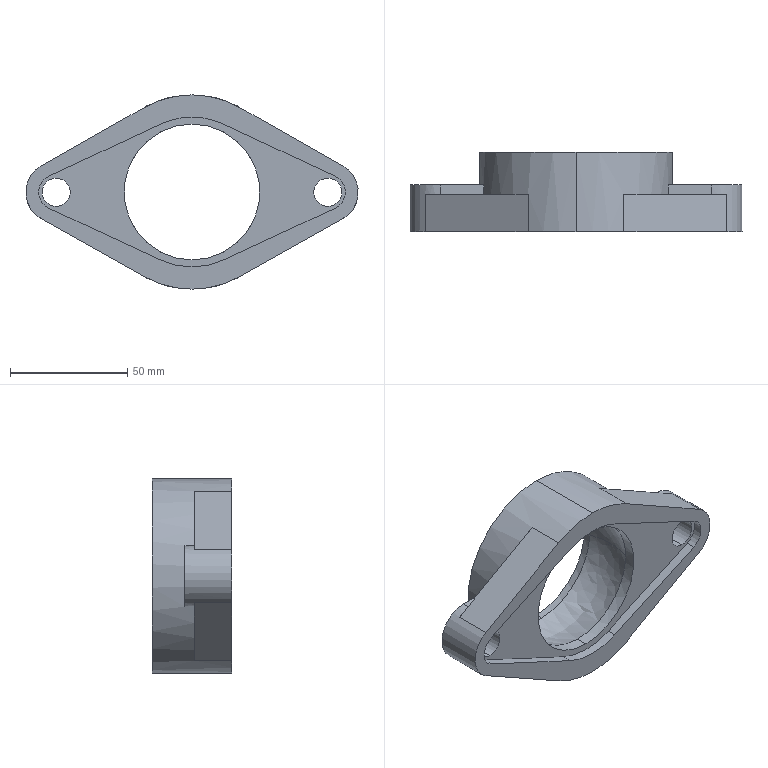Part | SolidWorks | features BaseBody 1 | 1 solid | 40 faces | box 142 x 34 x 83 mm | volume 116134 mm3 | plane 21 | cylinder 17 | spline 2 | commonest cylinder face diameters 12 x4 58 x4 64 x3 15 x2 26 x2 83 x2
STEP:
#1=CARTESIAN_POINT('',(31.,20.,0.));
#2=VERTEX_POINT('',#1);
#3=CARTESIAN_POINT('',(29.,30.954,0.));
#4=VERTEX_POINT('',#3);
#5=CARTESIAN_POINT('',(0.,20.,0.));
#6=DIRECTION('',(0.,0.,1.));
#7=DIRECTION('',(1.,0.,0.));
#8=AXIS2_PLACEMENT_3D('',#5,#6,#7);
#9=CIRCLE('',#8,31.);
#10=EDGE_CURVE('',#2,#4,#9,.T.);
#11=ORIENTED_EDGE('',*,*,#10,.F.);
#12=CARTESIAN_POINT('',(29.,9.046,0.));
#13=VERTEX_POINT('',#12);
#14=CARTESIAN_POINT('',(0.,20.,0.));
#15=DIRECTION('',(0.,0.,-1.));
#16=DIRECTION('',(1.,0.,0.));
#17=AXIS2_PLACEMENT_3D('',#14,#15,#16);
#18=CIRCLE('',#17,31.);
#19=EDGE_CURVE('',#2,#13,#18,.T.);
#20=ORIENTED_EDGE('',*,*,#19,.T.);
#21=CARTESIAN_POINT('',(0.,9.046,29.));
#22=VERTEX_POINT('',#21);
#23=CARTESIAN_POINT('',(0.,9.046,0.));
#24=DIRECTION('',(0.,1.,0.));
#25=DIRECTION('',(0.,0.,-1.));
#26=AXIS2_PLACEMENT_3D('',#23,#24,#25);
#27=CIRCLE('',#26,29.);
#28=EDGE_CURVE('',#22,#13,#27,.T.);
#29=ORIENTED_EDGE('',*,*,#28,.F.);
#30=CARTESIAN_POINT('',(-29.,9.046,0.));
#31=VERTEX_POINT('',#30);
#32=CARTESIAN_POINT('',(0.,9.046,0.));
#33=DIRECTION('',(0.,1.,0.));
#34=DIRECTION('',(0.,0.,-1.));
#35=AXIS2_PLACEMENT_3D('',#32,#33,#34);
#36=CIRCLE('',#35,29.);
#37=EDGE_CURVE('',#31,#22,#36,.T.);
#38=ORIENTED_EDGE('',*,*,#37,.F.);
#39=CARTESIAN_POINT('',(-31.,20.,0.));
#40=VERTEX_POINT('',#39);
#41=CARTESIAN_POINT('',(0.,20.,0.));
#42=DIRECTION('',(0.,0.,-1.));
#43=DIRECTION('',(1.,0.,0.));
#44=AXIS2_PLACEMENT_3D('',#41,#42,#43);
#45=CIRCLE('',#44,31.);
#46=EDGE_CURVE('',#31,#40,#45,.T.);
#47=ORIENTED_EDGE('',*,*,#46,.T.);
#48=CARTESIAN_POINT('',(-29.,30.954,0.));
#49=VERTEX_POINT('',#48);
#50=CARTESIAN_POINT('',(0.,20.,0.));
#51=DIRECTION('',(0.,0.,1.));
#52=DIRECTION('',(1.,0.,0.));
#53=AXIS2_PLACEMENT_3D('',#50,#51,#52);
#54=CIRCLE('',#53,31.);
#55=EDGE_CURVE('',#49,#40,#54,.T.);
#56=ORIENTED_EDGE('',*,*,#55,.F.);
#57=CARTESIAN_POINT('',(0.,30.954,29.));
#58=VERTEX_POINT('',#57);
#59=CARTESIAN_POINT('',(0.,30.954,0.));
#60=DIRECTION('',(0.,1.,0.));
#61=DIRECTION('',(0.,0.,-1.));
#62=AXIS2_PLACEMENT_3D('',#59,#60,#61);
#63=CIRCLE('',#62,29.);
#64=EDGE_CURVE('',#49,#58,#63,.T.);
#65=ORIENTED_EDGE('',*,*,#64,.T.);
#66=CARTESIAN_POINT('',(0.,30.954,0.));
#67=DIRECTION('',(0.,1.,0.));
#68=DIRECTION('',(0.,0.,-1.));
#69=AXIS2_PLACEMENT_3D('',#66,#67,#68);
#70=CIRCLE('',#69,29.);
#71=EDGE_CURVE('',#58,#4,#70,.T.);
#72=ORIENTED_EDGE('',*,*,#71,.T.);
#73=EDGE_LOOP('',(#11,#20,#29,#38,#47,#56,#65,#72));
#74=FACE_OUTER_BOUND('',#73,.T.);
#75=CARTESIAN_POINT('',(31.,20.,0.));
#76=CARTESIAN_POINT('',(31.,20.,0.));
#77=CARTESIAN_POINT('',(31.,20.,0.));
#78=CARTESIAN_POINT('',(31.,20.,0.));
#79=CARTESIAN_POINT('',(31.,82.,0.));
#80=CARTESIAN_POINT('',(31.,82.,124.));
#81=CARTESIAN_POINT('',(31.,-42.,124.));
#82=CARTESIAN_POINT('',(31.,-42.,0.));
#83=CARTESIAN_POINT('',(-31.,82.,0.));
#84=CARTESIAN_POINT('',(-31.,82.,124.));
#85=CARTESIAN_POINT('',(-31.,-42.,124.));
#86=CARTESIAN_POINT('',(-31.,-42.,0.));
#87=CARTESIAN_POINT('',(-31.,20.,0.));
#88=CARTESIAN_POINT('',(-31.,20.,0.));
#89=CARTESIAN_POINT('',(-31.,20.,0.));
#90=CARTESIAN_POINT('',(-31.,20.,0.));
#91=(BOUNDED_SURFACE()B_SPLINE_SURFACE(3,3,((#75,#76,#77,#78),(#79,#80,#81,#82),(#83,#84,#85,#86),(#87,#88,#89,#90)),.UNSPECIFIED.,.F.,.F.,.T.)B_SPLINE_SURFACE_WITH_KNOTS((4,4),(4,4),(0.,1.),(0.,1.),.UNSPECIFIED.)GEOMETRIC_REPRESENTATION_ITEM()RATIONAL_B_SPLINE_SURFACE(((1.,0.3333,0.3333,1.),(0.3333,0.1111,0.1111,0.3333),(0.3333,0.1111,0.1111,0.3333),(1.,0.3333,0.3333,1.)))REPRESENTATION_ITEM('')SURFACE());
#92=ADVANCED_FACE('',(#74),#91,.F.);
#93=CARTESIAN_POINT('',(20.327,0.,-36.181));
#94=VERTEX_POINT('',#93);
#95=CARTESIAN_POINT('',(0.,0.,-41.5));
#96=VERTEX_POINT('',#95);
#97=CARTESIAN_POINT('',(0.,0.,0.));
#98=DIRECTION('',(0.,1.,0.));
#99=DIRECTION('',(0.,0.,1.));
#100=AXIS2_PLACEMENT_3D('',#97,#98,#99);
#101=CIRCLE('',#100,41.5);
#102=EDGE_CURVE('',#94,#96,#101,.T.);
#103=ORIENTED_EDGE('',*,*,#102,.T.);
#104=CARTESIAN_POINT('',(0.,34.,-41.5));
#105=VERTEX_POINT('',#104);
#106=CARTESIAN_POINT('',(0.,0.,-41.5));
#107=DIRECTION('',(0.,1.,0.));
#108=VECTOR('',#107,1000.);
#109=LINE('',#106,#108);
#110=EDGE_CURVE('',#96,#105,#109,.T.);
#111=ORIENTED_EDGE('',*,*,#110,.T.);
#112=CARTESIAN_POINT('',(0.,34.,41.5));
#113=VERTEX_POINT('',#112);
#114=CARTESIAN_POINT('',(0.,34.,0.));
#115=DIRECTION('',(0.,-1.,0.));
#116=DIRECTION('',(0.,0.,1.));
#117=AXIS2_PLACEMENT_3D('',#114,#115,#116);
#118=CIRCLE('',#117,41.5);
#119=EDGE_CURVE('',#105,#113,#118,.T.);
#120=ORIENTED_EDGE('',*,*,#119,.T.);
#121=CARTESIAN_POINT('',(0.,0.,41.5));
#122=VERTEX_POINT('',#121);
#123=CARTESIAN_POINT('',(0.,0.,41.5));
#124=DIRECTION('',(0.,1.,0.));
#125=VECTOR('',#124,1000.);
#126=LINE('',#123,#125);
#127=EDGE_CURVE('',#122,#113,#126,.T.);
#128=ORIENTED_EDGE('',*,*,#127,.F.);
#129=CARTESIAN_POINT('',(20.458,0.,36.107));
#130=VERTEX_POINT('',#129);
#131=CARTESIAN_POINT('',(0.,0.,0.));
#132=DIRECTION('',(0.,1.,0.));
#133=DIRECTION('',(0.,0.,1.));
#134=AXIS2_PLACEMENT_3D('',#131,#132,#133);
#135=CIRCLE('',#134,41.5);
#136=EDGE_CURVE('',#122,#130,#135,.T.);
#137=ORIENTED_EDGE('',*,*,#136,.T.);
#138=CARTESIAN_POINT('',(20.458,16.,36.107));
#139=VERTEX_POINT('',#138);
#140=CARTESIAN_POINT('',(20.458,0.,36.107));
#141=DIRECTION('',(0.,1.,0.));
#142=VECTOR('',#141,1000.);
#143=LINE('',#140,#142);
#144=EDGE_CURVE('',#130,#139,#143,.T.);
#145=ORIENTED_EDGE('',*,*,#144,.T.);
#146=CARTESIAN_POINT('',(39.446,16.,12.895));
#147=VERTEX_POINT('',#146);
#148=CARTESIAN_POINT('',(0.,16.,0.));
#149=DIRECTION('',(0.,1.,0.));
#150=DIRECTION('',(0.,0.,1.));
#151=AXIS2_PLACEMENT_3D('',#148,#149,#150);
#152=CIRCLE('',#151,41.5);
#153=EDGE_CURVE('',#139,#147,#152,.T.);
#154=ORIENTED_EDGE('',*,*,#153,.T.);
#155=CARTESIAN_POINT('',(39.446,20.,12.895));
#156=VERTEX_POINT('',#155);
#157=CARTESIAN_POINT('',(39.446,0.,12.895));
#158=DIRECTION('',(0.,1.,0.));
#159=VECTOR('',#158,1000.);
#160=LINE('',#157,#159);
#161=EDGE_CURVE('',#147,#156,#160,.T.);
#162=ORIENTED_EDGE('',*,*,#161,.T.);
#163=CARTESIAN_POINT('',(39.376,20.,-13.105));
#164=VERTEX_POINT('',#163);
#165=CARTESIAN_POINT('',(0.,20.,0.));
#166=DIRECTION('',(0.,1.,0.));
#167=DIRECTION('',(0.,0.,1.));
#168=AXIS2_PLACEMENT_3D('',#165,#166,#167);
#169=CIRCLE('',#168,41.5);
#170=EDGE_CURVE('',#156,#164,#169,.T.);
#171=ORIENTED_EDGE('',*,*,#170,.T.);
#172=CARTESIAN_POINT('',(39.376,16.,-13.105));
#173=VERTEX_POINT('',#172);
#174=CARTESIAN_POINT('',(39.376,0.,-13.105));
#175=DIRECTION('',(0.,-1.,0.));
#176=VECTOR('',#175,1000.);
#177=LINE('',#174,#176);
#178=EDGE_CURVE('',#164,#173,#177,.T.);
#179=ORIENTED_EDGE('',*,*,#178,.T.);
#180=CARTESIAN_POINT('',(20.327,16.,-36.181));
#181=VERTEX_POINT('',#180);
#182=CARTESIAN_POINT('',(0.,16.,0.));
#183=DIRECTION('',(0.,1.,0.));
#184=DIRECTION('',(0.,0.,1.));
#185=AXIS2_PLACEMENT_3D('',#182,#183,#184);
#186=CIRCLE('',#185,41.5);
#187=EDGE_CURVE('',#173,#181,#186,.T.);
#188=ORIENTED_EDGE('',*,*,#187,.T.);
#189=CARTESIAN_POINT('',(20.327,0.,-36.181));
#190=DIRECTION('',(0.,-1.,0.));
#191=VECTOR('',#190,1000.);
#192=LINE('',#189,#191);
#193=EDGE_CURVE('',#181,#94,#192,.T.);
#194=ORIENTED_EDGE('',*,*,#193,.T.);
#195=EDGE_LOOP('',(#103,#111,#120,#128,#137,#145,#154,#162,#171,#179,#188,#194));
#196=FACE_OUTER_BOUND('',#195,.T.);
#197=CARTESIAN_POINT('',(0.,0.,0.));
#198=DIRECTION('',(0.,1.,0.));
#199=DIRECTION('',(0.,0.,1.));
#200=AXIS2_PLACEMENT_3D('',#197,#198,#199);
#201=CYLINDRICAL_SURFACE('',#200,41.5);
#202=ADVANCED_FACE('',(#196),#201,.T.);
#203=CARTESIAN_POINT('',(58.,4.,-6.105));
#204=VERTEX_POINT('',#203);
#205=CARTESIAN_POINT('',(58.,4.,5.895));
#206=VERTEX_POINT('',#205);
#207=CARTESIAN_POINT('',(58.,4.,-0.1052));
#208=DIRECTION('',(0.,1.,0.));
#209=DIRECTION('',(0.,0.,1.));
#210=AXIS2_PLACEMENT_3D('',#207,#208,#209);
#211=CIRCLE('',#210,6.);
#212=EDGE_CURVE('',#204,#206,#211,.T.);
#213=ORIENTED_EDGE('',*,*,#212,.F.);
#214=CARTESIAN_POINT('',(58.,20.,-6.105));
#215=VERTEX_POINT('',#214);
#216=CARTESIAN_POINT('',(58.,-147.955,-6.105));
#217=DIRECTION('',(0.,1.,0.));
#218=VECTOR('',#217,1000.);
#219=LINE('',#216,#218);
#220=EDGE_CURVE('',#204,#215,#219,.T.);
#221=ORIENTED_EDGE('',*,*,#220,.T.);
#222=CARTESIAN_POINT('',(58.,20.,5.895));
#223=VERTEX_POINT('',#222);
#224=CARTESIAN_POINT('',(58.,20.,-0.1052));
#225=DIRECTION('',(0.,1.,0.));
#226=DIRECTION('',(0.,0.,1.));
#227=AXIS2_PLACEMENT_3D('',#224,#225,#226);
#228=CIRCLE('',#227,6.);
#229=EDGE_CURVE('',#215,#223,#228,.T.);
#230=ORIENTED_EDGE('',*,*,#229,.T.);
#231=CARTESIAN_POINT('',(58.,-147.955,5.895));
#232=DIRECTION('',(0.,1.,0.));
#233=VECTOR('',#232,1000.);
#234=LINE('',#231,#233);
#235=EDGE_CURVE('',#206,#223,#234,.T.);
#236=ORIENTED_EDGE('',*,*,#235,.F.);
#237=EDGE_LOOP('',(#213,#221,#230,#236));
#238=FACE_OUTER_BOUND('',#237,.T.);
#239=CARTESIAN_POINT('',(58.,-147.955,-0.1052));
#240=DIRECTION('',(0.,1.,0.));
#241=DIRECTION('',(0.,0.,1.));
#242=AXIS2_PLACEMENT_3D('',#239,#240,#241);
#243=CYLINDRICAL_SURFACE('',#242,6.);
#244=ADVANCED_FACE('',(#238),#243,.F.);
#245=CARTESIAN_POINT('',(0.,0.,32.));
#246=VERTEX_POINT('',#245);
#247=CARTESIAN_POINT('',(13.57,0.,28.98));
#248=VERTEX_POINT('',#247);
#249=CARTESIAN_POINT('',(0.,0.,0.));
#250=DIRECTION('',(0.,1.,0.));
#251=DIRECTION('',(0.,0.,1.));
#252=AXIS2_PLACEMENT_3D('',#249,#250,#251);
#253=CIRCLE('',#252,32.);
#254=EDGE_CURVE('',#246,#248,#253,.T.);
#255=ORIENTED_EDGE('',*,*,#254,.F.);
#256=CARTESIAN_POINT('',(0.,4.,32.));
#257=VERTEX_POINT('',#256);
#258=CARTESIAN_POINT('',(0.,0.,32.));
#259=DIRECTION('',(0.,1.,0.));
#260=VECTOR('',#259,1000.);
#261=LINE('',#258,#260);
#262=EDGE_CURVE('',#246,#257,#261,.T.);
#263=ORIENTED_EDGE('',*,*,#262,.T.);
#264=CARTESIAN_POINT('',(13.57,4.,28.98));
#265=VERTEX_POINT('',#264);
#266=CARTESIAN_POINT('',(0.,4.,0.));
#267=DIRECTION('',(0.,-1.,0.));
#268=DIRECTION('',(0.,0.,1.));
#269=AXIS2_PLACEMENT_3D('',#266,#267,#268);
#270=CIRCLE('',#269,32.);
#271=EDGE_CURVE('',#265,#257,#270,.T.);
#272=ORIENTED_EDGE('',*,*,#271,.F.);
#273=CARTESIAN_POINT('',(13.57,0.,28.98));
#274=DIRECTION('',(0.,-1.,0.));
#275=VECTOR('',#274,1000.);
#276=LINE('',#273,#275);
#277=EDGE_CURVE('',#265,#248,#276,.T.);
#278=ORIENTED_EDGE('',*,*,#277,.T.);
#279=EDGE_LOOP('',(#255,#263,#272,#278));
#280=FACE_OUTER_BOUND('',#279,.T.);
#281=CARTESIAN_POINT('',(0.,0.,0.));
#282=DIRECTION('',(0.,1.,0.));
#283=DIRECTION('',(0.,0.,1.));
#284=AXIS2_PLACEMENT_3D('',#281,#282,#283);
#285=CYLINDRICAL_SURFACE('',#284,32.);
#286=ADVANCED_FACE('',(#280),#285,.F.);
#287=CARTESIAN_POINT('',(-58.,4.,-6.105));
#288=VERTEX_POINT('',#287);
#289=CARTESIAN_POINT('',(-58.,4.,5.895));
#290=VERTEX_POINT('',#289);
#291=CARTESIAN_POINT('',(-58.,4.,-0.1052));
#292=DIRECTION('',(0.,1.,0.));
#293=DIRECTION('',(0.,0.,1.));
#294=AXIS2_PLACEMENT_3D('',#291,#292,#293);
#295=CIRCLE('',#294,6.);
#296=EDGE_CURVE('',#288,#290,#295,.T.);
#297=ORIENTED_EDGE('',*,*,#296,.F.);
#298=CARTESIAN_POINT('',(-58.,20.,-6.105));
#299=VERTEX_POINT('',#298);
#300=CARTESIAN_POINT('',(-58.,-147.955,-6.105));
#301=DIRECTION('',(0.,1.,0.));
#302=VECTOR('',#301,1000.);
#303=LINE('',#300,#302);
#304=EDGE_CURVE('',#288,#299,#303,.T.);
#305=ORIENTED_EDGE('',*,*,#304,.T.);
#306=CARTESIAN_POINT('',(-58.,20.,5.895));
#307=VERTEX_POINT('',#306);
#308=CARTESIAN_POINT('',(-58.,20.,-0.1052));
#309=DIRECTION('',(0.,-1.,0.));
#310=DIRECTION('',(0.,0.,1.));
#311=AXIS2_PLACEMENT_3D('',#308,#309,#310);
#312=CIRCLE('',#311,6.);
#313=EDGE_CURVE('',#307,#299,#312,.T.);
#314=ORIENTED_EDGE('',*,*,#313,.F.);
#315=CARTESIAN_POINT('',(-58.,-147.955,5.895));
#316=DIRECTION('',(0.,1.,0.));
#317=VECTOR('',#316,1000.);
#318=LINE('',#315,#317);
#319=EDGE_CURVE('',#290,#307,#318,.T.);
#320=ORIENTED_EDGE('',*,*,#319,.F.);
#321=EDGE_LOOP('',(#297,#305,#314,#320));
#322=FACE_OUTER_BOUND('',#321,.T.);
#323=CARTESIAN_POINT('',(-58.,-147.955,-0.1052));
#324=DIRECTION('',(0.,1.,0.));
#325=DIRECTION('',(0.,0.,1.));
#326=AXIS2_PLACEMENT_3D('',#323,#324,#325);
#327=CYLINDRICAL_SURFACE('',#326,6.);
#328=ADVANCED_FACE('',(#322),#327,.F.);
#329=CARTESIAN_POINT('',(0.,34.,29.));
#330=VERTEX_POINT('',#329);
#331=CARTESIAN_POINT('',(0.,34.,-29.));
#332=VERTEX_POINT('',#331);
#333=CARTESIAN_POINT('',(0.,34.,0.));
#334=DIRECTION('',(0.,-1.,0.));
#335=DIRECTION('',(0.,0.,-1.));
#336=AXIS2_PLACEMENT_3D('',#333,#334,#335);
#337=CIRCLE('',#336,29.);
#338=EDGE_CURVE('',#330,#332,#337,.T.);
#339=ORIENTED_EDGE('',*,*,#338,.F.);
#340=CARTESIAN_POINT('',(0.,34.477,29.));
#341=DIRECTION('',(0.,-1.,0.));
#342=VECTOR('',#341,1000.);
#343=LINE('',#340,#342);
#344=EDGE_CURVE('',#330,#58,#343,.T.);
#345=ORIENTED_EDGE('',*,*,#344,.T.);
#346=ORIENTED_EDGE('',*,*,#64,.F.);
#347=CARTESIAN_POINT('',(0.,30.954,-29.));
#348=VERTEX_POINT('',#347);
#349=CARTESIAN_POINT('',(0.,30.954,0.));
#350=DIRECTION('',(0.,1.,0.));
#351=DIRECTION('',(0.,0.,-1.));
#352=AXIS2_PLACEMENT_3D('',#349,#350,#351);
#353=CIRCLE('',#352,29.);
#354=EDGE_CURVE('',#348,#49,#353,.T.);
#355=ORIENTED_EDGE('',*,*,#354,.F.);
#356=CARTESIAN_POINT('',(0.,34.477,-29.));
#357=DIRECTION('',(0.,-1.,0.));
#358=VECTOR('',#357,1000.);
#359=LINE('',#356,#358);
#360=EDGE_CURVE('',#332,#348,#359,.T.);
#361=ORIENTED_EDGE('',*,*,#360,.F.);
#362=EDGE_LOOP('',(#339,#345,#346,#355,#361));
#363=FACE_OUTER_BOUND('',#362,.T.);
#364=CARTESIAN_POINT('',(0.,34.477,0.));
#365=DIRECTION('',(0.,-1.,0.));
#366=DIRECTION('',(0.,0.,-1.));
#367=AXIS2_PLACEMENT_3D('',#364,#365,#366);
#368=CYLINDRICAL_SURFACE('',#367,29.);
#369=ADVANCED_FACE('',(#363),#368,.F.);
#370=CARTESIAN_POINT('',(0.,9.046,-29.));
#371=VERTEX_POINT('',#370);
#372=CARTESIAN_POINT('',(0.,9.046,0.));
#373=DIRECTION('',(0.,1.,0.));
#374=DIRECTION('',(0.,0.,-1.));
#375=AXIS2_PLACEMENT_3D('',#372,#373,#374);
#376=CIRCLE('',#375,29.);
#377=EDGE_CURVE('',#371,#31,#376,.T.);
#378=ORIENTED_EDGE('',*,*,#377,.T.);
#379=ORIENTED_EDGE('',*,*,#37,.T.);
#380=CARTESIAN_POINT('',(0.,4.,29.));
#381=VERTEX_POINT('',#380);
#382=CARTESIAN_POINT('',(0.,4.523,29.));
#383=DIRECTION('',(0.,-1.,0.));
#384=VECTOR('',#383,1000.);
#385=LINE('',#382,#384);
#386=EDGE_CURVE('',#22,#381,#385,.T.);
#387=ORIENTED_EDGE('',*,*,#386,.T.);
#388=CARTESIAN_POINT('',(0.,4.,-29.));
#389=VERTEX_POINT('',#388);
#390=CARTESIAN_POINT('',(0.,4.,0.));
#391=DIRECTION('',(0.,1.,0.));
#392=DIRECTION('',(0.,0.,-1.));
#393=AXIS2_PLACEMENT_3D('',#390,#391,#392);
#394=CIRCLE('',#393,29.);
#395=EDGE_CURVE('',#389,#381,#394,.T.);
#396=ORIENTED_EDGE('',*,*,#395,.F.);
#397=CARTESIAN_POINT('',(0.,4.523,-29.));
#398=DIRECTION('',(0.,-1.,0.));
#399=VECTOR('',#398,1000.);
#400=LINE('',#397,#399);
#401=EDGE_CURVE('',#371,#389,#400,.T.);
#402=ORIENTED_EDGE('',*,*,#401,.F.);
#403=EDGE_LOOP('',(#378,#379,#387,#396,#402));
#404=FACE_OUTER_BOUND('',#403,.T.);
#405=CARTESIAN_POINT('',(0.,4.523,0.));
#406=DIRECTION('',(0.,-1.,0.));
#407=DIRECTION('',(0.,0.,-1.));
#408=AXIS2_PLACEMENT_3D('',#405,#406,#407);
#409=CYLINDRICAL_SURFACE('',#408,29.);
#410=ADVANCED_FACE('',(#404),#409,.F.);
#411=ORIENTED_EDGE('',*,*,#110,.F.);
#412=CARTESIAN_POINT('',(-20.327,0.,-36.181));
#413=VERTEX_POINT('',#412);
#414=CARTESIAN_POINT('',(0.,0.,0.));
#415=DIRECTION('',(0.,1.,0.));
#416=DIRECTION('',(0.,0.,1.));
#417=AXIS2_PLACEMENT_3D('',#414,#415,#416);
#418=CIRCLE('',#417,41.5);
#419=EDGE_CURVE('',#96,#413,#418,.T.);
#420=ORIENTED_EDGE('',*,*,#419,.T.);
#421=CARTESIAN_POINT('',(-20.327,16.,-36.181));
#422=VERTEX_POINT('',#421);
#423=CARTESIAN_POINT('',(-20.327,0.,-36.181));
#424=DIRECTION('',(0.,1.,0.));
#425=VECTOR('',#424,1000.);
#426=LINE('',#423,#425);
#427=EDGE_CURVE('',#413,#422,#426,.T.);
#428=ORIENTED_EDGE('',*,*,#427,.T.);
#429=CARTESIAN_POINT('',(-39.376,16.,-13.105));
#430=VERTEX_POINT('',#429);
#431=CARTESIAN_POINT('',(0.,16.,0.));
#432=DIRECTION('',(0.,1.,0.));
#433=DIRECTION('',(0.,0.,1.));
#434=AXIS2_PLACEMENT_3D('',#431,#432,#433);
#435=CIRCLE('',#434,41.5);
#436=EDGE_CURVE('',#422,#430,#435,.T.);
#437=ORIENTED_EDGE('',*,*,#436,.T.);
#438=CARTESIAN_POINT('',(-39.376,20.,-13.105));
#439=VERTEX_POINT('',#438);
#440=CARTESIAN_POINT('',(-39.376,0.,-13.105));
#441=DIRECTION('',(0.,1.,0.));
#442=VECTOR('',#441,1000.);
#443=LINE('',#440,#442);
#444=EDGE_CURVE('',#430,#439,#443,.T.);
#445=ORIENTED_EDGE('',*,*,#444,.T.);
#446=CARTESIAN_POINT('',(-39.446,20.,12.895));
#447=VERTEX_POINT('',#446);
#448=CARTESIAN_POINT('',(0.,20.,0.));
#449=DIRECTION('',(0.,1.,0.));
#450=DIRECTION('',(0.,0.,1.));
#451=AXIS2_PLACEMENT_3D('',#448,#449,#450);
#452=CIRCLE('',#451,41.5);
#453=EDGE_CURVE('',#439,#447,#452,.T.);
#454=ORIENTED_EDGE('',*,*,#453,.T.);
#455=CARTESIAN_POINT('',(-39.446,16.,12.895));
#456=VERTEX_POINT('',#455);
#457=CARTESIAN_POINT('',(-39.446,0.,12.895));
#458=DIRECTION('',(0.,-1.,0.));
#459=VECTOR('',#458,1000.);
#460=LINE('',#457,#459);
#461=EDGE_CURVE('',#447,#456,#460,.T.);
#462=ORIENTED_EDGE('',*,*,#461,.T.);
#463=CARTESIAN_POINT('',(-20.458,16.,36.107));
#464=VERTEX_POINT('',#463);
#465=CARTESIAN_POINT('',(0.,16.,0.));
#466=DIRECTION('',(0.,1.,0.));
#467=DIRECTION('',(0.,0.,1.));
#468=AXIS2_PLACEMENT_3D('',#465,#466,#467);
#469=CIRCLE('',#468,41.5);
#470=EDGE_CURVE('',#456,#464,#469,.T.);
#471=ORIENTED_EDGE('',*,*,#470,.T.);
#472=CARTESIAN_POINT('',(-20.458,0.,36.107));
#473=VERTEX_POINT('',#472);
#474=CARTESIAN_POINT('',(-20.458,0.,36.107));
#475=DIRECTION('',(0.,-1.,0.));
#476=VECTOR('',#475,1000.);
#477=LINE('',#474,#476);
#478=EDGE_CURVE('',#464,#473,#477,.T.);
#479=ORIENTED_EDGE('',*,*,#478,.T.);
#480=CARTESIAN_POINT('',(0.,0.,0.));
#481=DIRECTION('',(0.,1.,0.));
#482=DIRECTION('',(0.,0.,1.));
#483=AXIS2_PLACEMENT_3D('',#480,#481,#482);
#484=CIRCLE('',#483,41.5);
#485=EDGE_CURVE('',#473,#122,#484,.T.);
#486=ORIENTED_EDGE('',*,*,#485,.T.);
#487=ORIENTED_EDGE('',*,*,#127,.T.);
#488=CARTESIAN_POINT('',(0.,34.,0.));
#489=DIRECTION('',(0.,-1.,0.));
#490=DIRECTION('',(0.,0.,1.));
#491=AXIS2_PLACEMENT_3D('',#488,#489,#490);
#492=CIRCLE('',#491,41.5);
#493=EDGE_CURVE('',#113,#105,#492,.T.);
#494=ORIENTED_EDGE('',*,*,#493,.T.);
#495=EDGE_LOOP('',(#411,#420,#428,#437,#445,#454,#462,#471,#479,#486,#487,#494));
#496=FACE_OUTER_BOUND('',#495,.T.);
#497=CARTESIAN_POINT('',(0.,0.,0.));
#498=DIRECTION('',(0.,1.,0.));
#499=DIRECTION('',(0.,0.,1.));
#500=AXIS2_PLACEMENT_3D('',#497,#498,#499);
#501=CYLINDRICAL_SURFACE('',#500,41.5);
#502=ADVANCED_FACE('',(#496),#501,.T.);
#503=CARTESIAN_POINT('',(64.367,16.,-11.439));
#504=VERTEX_POINT('',#503);
#505=CARTESIAN_POINT('',(64.367,16.,-11.439));
#506=DIRECTION('',(0.8718,0.,0.4898));
#507=VECTOR('',#506,1000.);
#508=LINE('',#505,#507);
#509=EDGE_CURVE('',#181,#504,#508,.T.);
#510=ORIENTED_EDGE('',*,*,#509,.T.);
#511=CARTESIAN_POINT('',(64.367,0.,-11.439));
#512=VERTEX_POINT('',#511);
#513=CARTESIAN_POINT('',(64.367,0.,-11.439));
#514=DIRECTION('',(0.,-1.,0.));
#515=VECTOR('',#514,1000.);
#516=LINE('',#513,#515);
#517=EDGE_CURVE('',#504,#512,#516,.T.);
#518=ORIENTED_EDGE('',*,*,#517,.T.);
#519=CARTESIAN_POINT('',(64.367,0.,-11.439));
#520=DIRECTION('',(-0.8718,0.,-0.4898));
#521=VECTOR('',#520,1000.);
#522=LINE('',#519,#521);
#523=EDGE_CURVE('',#512,#94,#522,.T.);
#524=ORIENTED_EDGE('',*,*,#523,.T.);
#525=ORIENTED_EDGE('',*,*,#193,.F.);
#526=EDGE_LOOP('',(#510,#518,#524,#525));
#527=FACE_OUTER_BOUND('',#526,.T.);
#528=CARTESIAN_POINT('',(64.367,0.,-11.439));
#529=DIRECTION('',(0.4898,0.,-0.8718));
#530=DIRECTION('',(-0.8718,0.,-0.4898));
#531=AXIS2_PLACEMENT_3D('',#528,#529,#530);
#532=PLANE('',#531);
#533=ADVANCED_FACE('',(#527),#532,.T.);
#534=CARTESIAN_POINT('',(58.,16.,-13.105));
#535=VERTEX_POINT('',#534);
#536=CARTESIAN_POINT('',(-0.00009009,16.,-13.105));
#537=DIRECTION('',(-1.,0.,0.));
#538=VECTOR('',#537,1000.);
#539=LINE('',#536,#538);
#540=EDGE_CURVE('',#535,#173,#539,.T.);
#541=ORIENTED_EDGE('',*,*,#540,.F.);
#542=CARTESIAN_POINT('',(58.,16.,-0.1052));
#543=DIRECTION('',(0.,1.,0.));
#544=DIRECTION('',(0.,0.,1.));
#545=AXIS2_PLACEMENT_3D('',#542,#543,#544);
#546=CIRCLE('',#545,13.);
#547=EDGE_CURVE('',#504,#535,#546,.T.);
#548=ORIENTED_EDGE('',*,*,#547,.F.);
#549=ORIENTED_EDGE('',*,*,#509,.F.);
#550=ORIENTED_EDGE('',*,*,#187,.F.);
#551=EDGE_LOOP('',(#541,#548,#549,#550));
#552=FACE_OUTER_BOUND('',#551,.T.);
#553=CARTESIAN_POINT('',(-0.00009009,16.,-0.04073));
#554=DIRECTION('',(0.,-1.,0.));
#555=DIRECTION('',(0.,0.,-1.));
#556=AXIS2_PLACEMENT_3D('',#553,#554,#555);
#557=PLANE('',#556);
#558=ADVANCED_FACE('',(#552),#557,.F.);
#559=CARTESIAN_POINT('',(58.,20.,-13.105));
#560=VERTEX_POINT('',#559);
#561=CARTESIAN_POINT('',(58.,20.,-13.105));
#562=DIRECTION('',(1.,0.,0.));
#563=VECTOR('',#562,1000.);
#564=LINE('',#561,#563);
#565=EDGE_CURVE('',#164,#560,#564,.T.);
#566=ORIENTED_EDGE('',*,*,#565,.T.);
#567=CARTESIAN_POINT('',(58.,16.,-13.105));
#568=DIRECTION('',(0.,-1.,0.));
#569=VECTOR('',#568,1000.);
#570=LINE('',#567,#569);
#571=EDGE_CURVE('',#560,#535,#570,.T.);
#572=ORIENTED_EDGE('',*,*,#571,.T.);
#573=ORIENTED_EDGE('',*,*,#540,.T.);
#574=ORIENTED_EDGE('',*,*,#178,.F.);
#575=EDGE_LOOP('',(#566,#572,#573,#574));
#576=FACE_OUTER_BOUND('',#575,.T.);
#577=CARTESIAN_POINT('',(58.,16.,-13.105));
#578=DIRECTION('',(0.,0.,-1.));
#579=DIRECTION('',(-1.,0.,0.));
#580=AXIS2_PLACEMENT_3D('',#577,#578,#579);
#581=PLANE('',#580);
#582=ADVANCED_FACE('',(#576),#581,.T.);
#583=CARTESIAN_POINT('',(58.,20.,-0.1052));
#584=DIRECTION('',(0.,1.,0.));
#585=DIRECTION('',(0.,0.,1.));
#586=AXIS2_PLACEMENT_3D('',#583,#584,#585);
#587=CIRCLE('',#586,6.);
#588=EDGE_CURVE('',#223,#215,#587,.T.);
#589=ORIENTED_EDGE('',*,*,#588,.F.);
#590=ORIENTED_EDGE('',*,*,#229,.F.);
#591=EDGE_LOOP('',(#589,#590));
#592=FACE_BOUND('',#591,.T.);
#593=ORIENTED_EDGE('',*,*,#170,.F.);
#594=CARTESIAN_POINT('',(58.,20.,12.895));
#595=VERTEX_POINT('',#594);
#596=CARTESIAN_POINT('',(53.058,20.,12.895));
#597=DIRECTION('',(-1.,0.,0.));
#598=VECTOR('',#597,1000.);
#599=LINE('',#596,#598);
#600=EDGE_CURVE('',#595,#156,#599,.T.);
#601=ORIENTED_EDGE('',*,*,#600,.F.);
#602=CARTESIAN_POINT('',(58.,20.,-0.1052));
#603=DIRECTION('',(0.,-1.,0.));
#604=DIRECTION('',(0.,0.,1.));
#605=AXIS2_PLACEMENT_3D('',#602,#603,#604);
#606=CIRCLE('',#605,13.);
#607=EDGE_CURVE('',#560,#595,#606,.T.);
#608=ORIENTED_EDGE('',*,*,#607,.F.);
#609=ORIENTED_EDGE('',*,*,#565,.F.);
#610=EDGE_LOOP('',(#593,#601,#608,#609));
#611=FACE_OUTER_BOUND('',#610,.T.);
#612=CARTESIAN_POINT('',(53.058,20.,-0.1164));
#613=DIRECTION('',(0.,-1.,0.));
#614=DIRECTION('',(0.,0.,-1.));
#615=AXIS2_PLACEMENT_3D('',#612,#613,#614);
#616=PLANE('',#615);
#617=ADVANCED_FACE('',(#592,#611),#616,.F.);
#618=ORIENTED_EDGE('',*,*,#600,.T.);
#619=ORIENTED_EDGE('',*,*,#161,.F.);
#620=CARTESIAN_POINT('',(58.,16.,12.895));
#621=VERTEX_POINT('',#620);
#622=CARTESIAN_POINT('',(39.446,16.,12.895));
#623=DIRECTION('',(1.,0.,0.));
#624=VECTOR('',#623,1000.);
#625=LINE('',#622,#624);
#626=EDGE_CURVE('',#147,#621,#625,.T.);
#627=ORIENTED_EDGE('',*,*,#626,.T.);
#628=CARTESIAN_POINT('',(58.,16.,12.895));
#629=DIRECTION('',(0.,1.,0.));
#630=VECTOR('',#629,1000.);
#631=LINE('',#628,#630);
#632=EDGE_CURVE('',#621,#595,#631,.T.);
#633=ORIENTED_EDGE('',*,*,#632,.T.);
#634=EDGE_LOOP('',(#618,#619,#627,#633));
#635=FACE_OUTER_BOUND('',#634,.T.);
#636=CARTESIAN_POINT('',(39.446,16.,12.895));
#637=DIRECTION('',(0.,0.,1.));
#638=DIRECTION('',(1.,0.,0.));
#639=AXIS2_PLACEMENT_3D('',#636,#637,#638);
#640=PLANE('',#639);
#641=ADVANCED_FACE('',(#635),#640,.T.);
#642=CARTESIAN_POINT('',(64.408,16.,11.205));
#643=VERTEX_POINT('',#642);
#644=CARTESIAN_POINT('',(64.408,16.,11.205));
#645=DIRECTION('',(-0.8701,0.,0.493));
#646=VECTOR('',#645,1000.);
#647=LINE('',#644,#646);
#648=EDGE_CURVE('',#643,#139,#647,.T.);
#649=ORIENTED_EDGE('',*,*,#648,.F.);
#650=CARTESIAN_POINT('',(58.,16.,-0.1052));
#651=DIRECTION('',(0.,1.,0.));
#652=DIRECTION('',(0.,0.,1.));
#653=AXIS2_PLACEMENT_3D('',#650,#651,#652);
#654=CIRCLE('',#653,13.);
#655=EDGE_CURVE('',#621,#643,#654,.T.);
#656=ORIENTED_EDGE('',*,*,#655,.F.);
#657=ORIENTED_EDGE('',*,*,#626,.F.);
#658=ORIENTED_EDGE('',*,*,#153,.F.);
#659=EDGE_LOOP('',(#649,#656,#657,#658));
#660=FACE_OUTER_BOUND('',#659,.T.);
#661=CARTESIAN_POINT('',(-0.00009009,16.,-0.04073));
#662=DIRECTION('',(0.,-1.,0.));
#663=DIRECTION('',(0.,0.,-1.));
#664=AXIS2_PLACEMENT_3D('',#661,#662,#663);
#665=PLANE('',#664);
#666=ADVANCED_FACE('',(#660),#665,.F.);
#667=ORIENTED_EDGE('',*,*,#648,.T.);
#668=ORIENTED_EDGE('',*,*,#144,.F.);
#669=CARTESIAN_POINT('',(64.408,0.,11.205));
#670=VERTEX_POINT('',#669);
#671=CARTESIAN_POINT('',(20.458,0.,36.107));
#672=DIRECTION('',(0.8701,0.,-0.493));
#673=VECTOR('',#672,1000.);
#674=LINE('',#671,#673);
#675=EDGE_CURVE('',#130,#670,#674,.T.);
#676=ORIENTED_EDGE('',*,*,#675,.T.);
#677=CARTESIAN_POINT('',(64.408,0.,11.205));
#678=DIRECTION('',(0.,1.,0.));
#679=VECTOR('',#678,1000.);
#680=LINE('',#677,#679);
#681=EDGE_CURVE('',#670,#643,#680,.T.);
#682=ORIENTED_EDGE('',*,*,#681,.T.);
#683=EDGE_LOOP('',(#667,#668,#676,#682));
#684=FACE_OUTER_BOUND('',#683,.T.);
#685=CARTESIAN_POINT('',(20.458,0.,36.107));
#686=DIRECTION('',(0.493,0.,0.8701));
#687=DIRECTION('',(0.8701,0.,-0.493));
#688=AXIS2_PLACEMENT_3D('',#685,#686,#687);
#689=PLANE('',#688);
#690=ADVANCED_FACE('',(#684),#689,.T.);
#691=CARTESIAN_POINT('',(61.156,0.,-6.909));
#692=VERTEX_POINT('',#691);
#693=CARTESIAN_POINT('',(13.465,0.,-29.029));
#694=VERTEX_POINT('',#693);
#695=CARTESIAN_POINT('',(61.156,0.,-6.909));
#696=DIRECTION('',(-0.9072,0.,-0.4208));
#697=VECTOR('',#696,1000.);
#698=LINE('',#695,#697);
#699=EDGE_CURVE('',#692,#694,#698,.T.);
#700=ORIENTED_EDGE('',*,*,#699,.T.);
#701=CARTESIAN_POINT('',(-13.465,0.,-29.029));
#702=VERTEX_POINT('',#701);
#703=CARTESIAN_POINT('',(0.,0.,0.));
#704=DIRECTION('',(0.,1.,0.));
#705=DIRECTION('',(0.,0.,1.));
#706=AXIS2_PLACEMENT_3D('',#703,#704,#705);
#707=CIRCLE('',#706,32.);
#708=EDGE_CURVE('',#694,#702,#707,.T.);
#709=ORIENTED_EDGE('',*,*,#708,.T.);
#710=CARTESIAN_POINT('',(-61.156,0.,-6.909));
#711=VERTEX_POINT('',#710);
#712=CARTESIAN_POINT('',(-13.465,0.,-29.029));
#713=DIRECTION('',(-0.9072,0.,0.4208));
#714=VECTOR('',#713,1000.);
#715=LINE('',#712,#714);
#716=EDGE_CURVE('',#702,#711,#715,.T.);
#717=ORIENTED_EDGE('',*,*,#716,.T.);
#718=CARTESIAN_POINT('',(-61.181,0.,6.687));
#719=VERTEX_POINT('',#718);
#720=CARTESIAN_POINT('',(-58.,0.,-0.1052));
#721=DIRECTION('',(0.,1.,0.));
#722=DIRECTION('',(0.,0.,1.));
#723=AXIS2_PLACEMENT_3D('',#720,#721,#722);
#724=CIRCLE('',#723,7.5);
#725=EDGE_CURVE('',#711,#719,#724,.T.);
#726=ORIENTED_EDGE('',*,*,#725,.T.);
#727=CARTESIAN_POINT('',(-13.57,0.,28.98));
#728=VERTEX_POINT('',#727);
#729=CARTESIAN_POINT('',(-61.181,0.,6.687));
#730=DIRECTION('',(0.9056,0.,0.4241));
#731=VECTOR('',#730,1000.);
#732=LINE('',#729,#731);
#733=EDGE_CURVE('',#719,#728,#732,.T.);
#734=ORIENTED_EDGE('',*,*,#733,.T.);
#735=CARTESIAN_POINT('',(0.,0.,0.));
#736=DIRECTION('',(0.,1.,0.));
#737=DIRECTION('',(0.,0.,1.));
#738=AXIS2_PLACEMENT_3D('',#735,#736,#737);
#739=CIRCLE('',#738,32.);
#740=EDGE_CURVE('',#728,#246,#739,.T.);
#741=ORIENTED_EDGE('',*,*,#740,.T.);
#742=ORIENTED_EDGE('',*,*,#254,.T.);
#743=CARTESIAN_POINT('',(61.18,0.,6.687));
#744=VERTEX_POINT('',#743);
#745=CARTESIAN_POINT('',(13.57,0.,28.98));
#746=DIRECTION('',(0.9056,0.,-0.4241));
#747=VECTOR('',#746,1000.);
#748=LINE('',#745,#747);
#749=EDGE_CURVE('',#248,#744,#748,.T.);
#750=ORIENTED_EDGE('',*,*,#749,.T.);
#751=CARTESIAN_POINT('',(58.,0.,-0.1052));
#752=DIRECTION('',(0.,1.,0.));
#753=DIRECTION('',(0.,0.,1.));
#754=AXIS2_PLACEMENT_3D('',#751,#752,#753);
#755=CIRCLE('',#754,7.5);
#756=EDGE_CURVE('',#744,#692,#755,.T.);
#757=ORIENTED_EDGE('',*,*,#756,.T.);
#758=EDGE_LOOP('',(#700,#709,#717,#726,#734,#741,#742,#750,#757));
#759=FACE_BOUND('',#758,.T.);
#760=ORIENTED_EDGE('',*,*,#102,.F.);
#761=ORIENTED_EDGE('',*,*,#523,.F.);
#762=CARTESIAN_POINT('',(58.,0.,-0.1052));
#763=DIRECTION('',(0.,-1.,0.));
#764=DIRECTION('',(0.,0.,1.));
#765=AXIS2_PLACEMENT_3D('',#762,#763,#764);
#766=CIRCLE('',#765,13.);
#767=EDGE_CURVE('',#512,#670,#766,.T.);
#768=ORIENTED_EDGE('',*,*,#767,.T.);
#769=ORIENTED_EDGE('',*,*,#675,.F.);
#770=ORIENTED_EDGE('',*,*,#136,.F.);
#771=ORIENTED_EDGE('',*,*,#485,.F.);
#772=CARTESIAN_POINT('',(-64.409,0.,11.205));
#773=VERTEX_POINT('',#772);
#774=CARTESIAN_POINT('',(-20.458,0.,36.107));
#775=DIRECTION('',(-0.8701,0.,-0.493));
#776=VECTOR('',#775,1000.);
#777=LINE('',#774,#776);
#778=EDGE_CURVE('',#473,#773,#777,.T.);
#779=ORIENTED_EDGE('',*,*,#778,.T.);
#780=CARTESIAN_POINT('',(-64.367,0.,-11.439));
#781=VERTEX_POINT('',#780);
#782=CARTESIAN_POINT('',(-58.,0.,-0.1052));
#783=DIRECTION('',(0.,-1.,0.));
#784=DIRECTION('',(0.,0.,1.));
#785=AXIS2_PLACEMENT_3D('',#782,#783,#784);
#786=CIRCLE('',#785,13.);
#787=EDGE_CURVE('',#773,#781,#786,.T.);
#788=ORIENTED_EDGE('',*,*,#787,.T.);
#789=CARTESIAN_POINT('',(-64.367,0.,-11.439));
#790=DIRECTION('',(0.8718,0.,-0.4898));
#791=VECTOR('',#790,1000.);
#792=LINE('',#789,#791);
#793=EDGE_CURVE('',#781,#413,#792,.T.);
#794=ORIENTED_EDGE('',*,*,#793,.T.);
#795=ORIENTED_EDGE('',*,*,#419,.F.);
#796=EDGE_LOOP('',(#760,#761,#768,#769,#770,#771,#779,#788,#794,#795));
#797=FACE_OUTER_BOUND('',#796,.T.);
#798=CARTESIAN_POINT('',(-0.00009009,0.,-0.04073));
#799=DIRECTION('',(0.,-1.,0.));
#800=DIRECTION('',(0.,0.,-1.));
#801=AXIS2_PLACEMENT_3D('',#798,#799,#800);
#802=PLANE('',#801);
#803=ADVANCED_FACE('',(#759,#797),#802,.T.);
#804=CARTESIAN_POINT('',(-64.409,16.,11.205));
#805=VERTEX_POINT('',#804);
#806=CARTESIAN_POINT('',(-64.409,16.,11.205));
#807=DIRECTION('',(-0.8701,0.,-0.493));
#808=VECTOR('',#807,1000.);
#809=LINE('',#806,#808);
#810=EDGE_CURVE('',#464,#805,#809,.T.);
#811=ORIENTED_EDGE('',*,*,#810,.T.);
#812=CARTESIAN_POINT('',(-64.409,0.,11.205));
#813=DIRECTION('',(0.,-1.,0.));
#814=VECTOR('',#813,1000.);
#815=LINE('',#812,#814);
#816=EDGE_CURVE('',#805,#773,#815,.T.);
#817=ORIENTED_EDGE('',*,*,#816,.T.);
#818=ORIENTED_EDGE('',*,*,#778,.F.);
#819=ORIENTED_EDGE('',*,*,#478,.F.);
#820=EDGE_LOOP('',(#811,#817,#818,#819));
#821=FACE_OUTER_BOUND('',#820,.T.);
#822=CARTESIAN_POINT('',(-64.409,0.,11.205));
#823=DIRECTION('',(-0.493,0.,0.8701));
#824=DIRECTION('',(0.8701,0.,0.493));
#825=AXIS2_PLACEMENT_3D('',#822,#823,#824);
#826=PLANE('',#825);
#827=ADVANCED_FACE('',(#821),#826,.T.);
#828=CARTESIAN_POINT('',(-58.,16.,12.895));
#829=VERTEX_POINT('',#828);
#830=CARTESIAN_POINT('',(-0.00009009,16.,12.895));
#831=DIRECTION('',(1.,0.,0.));
#832=VECTOR('',#831,1000.);
#833=LINE('',#830,#832);
#834=EDGE_CURVE('',#829,#456,#833,.T.);
#835=ORIENTED_EDGE('',*,*,#834,.F.);
#836=CARTESIAN_POINT('',(-58.,16.,-0.1052));
#837=DIRECTION('',(0.,1.,0.));
#838=DIRECTION('',(0.,0.,1.));
#839=AXIS2_PLACEMENT_3D('',#836,#837,#838);
#840=CIRCLE('',#839,13.);
#841=EDGE_CURVE('',#805,#829,#840,.T.);
#842=ORIENTED_EDGE('',*,*,#841,.F.);
#843=ORIENTED_EDGE('',*,*,#810,.F.);
#844=ORIENTED_EDGE('',*,*,#470,.F.);
#845=EDGE_LOOP('',(#835,#842,#843,#844));
#846=FACE_OUTER_BOUND('',#845,.T.);
#847=CARTESIAN_POINT('',(-0.00009009,16.,-0.04073));
#848=DIRECTION('',(0.,-1.,0.));
#849=DIRECTION('',(0.,0.,-1.));
#850=AXIS2_PLACEMENT_3D('',#847,#848,#849);
#851=PLANE('',#850);
#852=ADVANCED_FACE('',(#846),#851,.F.);
#853=CARTESIAN_POINT('',(-58.,20.,12.895));
#854=VERTEX_POINT('',#853);
#855=CARTESIAN_POINT('',(-58.,20.,12.895));
#856=DIRECTION('',(-1.,0.,0.));
#857=VECTOR('',#856,1000.);
#858=LINE('',#855,#857);
#859=EDGE_CURVE('',#447,#854,#858,.T.);
#860=ORIENTED_EDGE('',*,*,#859,.T.);
#861=CARTESIAN_POINT('',(-58.,16.,12.895));
#862=DIRECTION('',(0.,-1.,0.));
#863=VECTOR('',#862,1000.);
#864=LINE('',#861,#863);
#865=EDGE_CURVE('',#854,#829,#864,.T.);
#866=ORIENTED_EDGE('',*,*,#865,.T.);
#867=ORIENTED_EDGE('',*,*,#834,.T.);
#868=ORIENTED_EDGE('',*,*,#461,.F.);
#869=EDGE_LOOP('',(#860,#866,#867,#868));
#870=FACE_OUTER_BOUND('',#869,.T.);
#871=CARTESIAN_POINT('',(-58.,16.,12.895));
#872=DIRECTION('',(0.,0.,1.));
#873=DIRECTION('',(1.,0.,0.));
#874=AXIS2_PLACEMENT_3D('',#871,#872,#873);
#875=PLANE('',#874);
#876=ADVANCED_FACE('',(#870),#875,.T.);
#877=ORIENTED_EDGE('',*,*,#313,.T.);
#878=CARTESIAN_POINT('',(-58.,20.,-0.1052));
#879=DIRECTION('',(0.,-1.,0.));
#880=DIRECTION('',(0.,0.,1.));
#881=AXIS2_PLACEMENT_3D('',#878,#879,#880);
#882=CIRCLE('',#881,6.);
#883=EDGE_CURVE('',#299,#307,#882,.T.);
#884=ORIENTED_EDGE('',*,*,#883,.T.);
#885=EDGE_LOOP('',(#877,#884));
#886=FACE_BOUND('',#885,.T.);
#887=ORIENTED_EDGE('',*,*,#453,.F.);
#888=CARTESIAN_POINT('',(-58.,20.,-13.105));
#889=VERTEX_POINT('',#888);
#890=CARTESIAN_POINT('',(-53.058,20.,-13.105));
#891=DIRECTION('',(-1.,0.,0.));
#892=VECTOR('',#891,1000.);
#893=LINE('',#890,#892);
#894=EDGE_CURVE('',#439,#889,#893,.T.);
#895=ORIENTED_EDGE('',*,*,#894,.T.);
#896=CARTESIAN_POINT('',(-58.,20.,-0.1052));
#897=DIRECTION('',(0.,1.,0.));
#898=DIRECTION('',(0.,0.,1.));
#899=AXIS2_PLACEMENT_3D('',#896,#897,#898);
#900=CIRCLE('',#899,13.);
#901=EDGE_CURVE('',#889,#854,#900,.T.);
#902=ORIENTED_EDGE('',*,*,#901,.T.);
#903=ORIENTED_EDGE('',*,*,#859,.F.);
#904=EDGE_LOOP('',(#887,#895,#902,#903));
#905=FACE_OUTER_BOUND('',#904,.T.);
#906=CARTESIAN_POINT('',(-53.058,20.,-0.1164));
#907=DIRECTION('',(0.,1.,0.));
#908=DIRECTION('',(0.,0.,1.));
#909=AXIS2_PLACEMENT_3D('',#906,#907,#908);
#910=PLANE('',#909);
#911=ADVANCED_FACE('',(#886,#905),#910,.T.);
#912=ORIENTED_EDGE('',*,*,#894,.F.);
#913=ORIENTED_EDGE('',*,*,#444,.F.);
#914=CARTESIAN_POINT('',(-58.,16.,-13.105));
#915=VERTEX_POINT('',#914);
#916=CARTESIAN_POINT('',(-39.376,16.,-13.105));
#917=DIRECTION('',(-1.,0.,0.));
#918=VECTOR('',#917,1000.);
#919=LINE('',#916,#918);
#920=EDGE_CURVE('',#430,#915,#919,.T.);
#921=ORIENTED_EDGE('',*,*,#920,.T.);
#922=CARTESIAN_POINT('',(-58.,16.,-13.105));
#923=DIRECTION('',(0.,1.,0.));
#924=VECTOR('',#923,1000.);
#925=LINE('',#922,#924);
#926=EDGE_CURVE('',#915,#889,#925,.T.);
#927=ORIENTED_EDGE('',*,*,#926,.T.);
#928=EDGE_LOOP('',(#912,#913,#921,#927));
#929=FACE_OUTER_BOUND('',#928,.T.);
#930=CARTESIAN_POINT('',(-39.376,16.,-13.105));
#931=DIRECTION('',(0.,0.,-1.));
#932=DIRECTION('',(-1.,0.,0.));
#933=AXIS2_PLACEMENT_3D('',#930,#931,#932);
#934=PLANE('',#933);
#935=ADVANCED_FACE('',(#929),#934,.T.);
#936=CARTESIAN_POINT('',(-64.367,16.,-11.439));
#937=VERTEX_POINT('',#936);
#938=CARTESIAN_POINT('',(-64.367,16.,-11.439));
#939=DIRECTION('',(0.8718,0.,-0.4898));
#940=VECTOR('',#939,1000.);
#941=LINE('',#938,#940);
#942=EDGE_CURVE('',#937,#422,#941,.T.);
#943=ORIENTED_EDGE('',*,*,#942,.F.);
#944=CARTESIAN_POINT('',(-58.,16.,-0.1052));
#945=DIRECTION('',(0.,1.,0.));
#946=DIRECTION('',(0.,0.,1.));
#947=AXIS2_PLACEMENT_3D('',#944,#945,#946);
#948=CIRCLE('',#947,13.);
#949=EDGE_CURVE('',#915,#937,#948,.T.);
#950=ORIENTED_EDGE('',*,*,#949,.F.);
#951=ORIENTED_EDGE('',*,*,#920,.F.);
#952=ORIENTED_EDGE('',*,*,#436,.F.);
#953=EDGE_LOOP('',(#943,#950,#951,#952));
#954=FACE_OUTER_BOUND('',#953,.T.);
#955=CARTESIAN_POINT('',(-0.00009009,16.,-0.04073));
#956=DIRECTION('',(0.,-1.,0.));
#957=DIRECTION('',(0.,0.,-1.));
#958=AXIS2_PLACEMENT_3D('',#955,#956,#957);
#959=PLANE('',#958);
#960=ADVANCED_FACE('',(#954),#959,.F.);
#961=ORIENTED_EDGE('',*,*,#942,.T.);
#962=ORIENTED_EDGE('',*,*,#427,.F.);
#963=ORIENTED_EDGE('',*,*,#793,.F.);
#964=CARTESIAN_POINT('',(-64.367,0.,-11.439));
#965=DIRECTION('',(0.,1.,0.));
#966=VECTOR('',#965,1000.);
#967=LINE('',#964,#966);
#968=EDGE_CURVE('',#781,#937,#967,.T.);
#969=ORIENTED_EDGE('',*,*,#968,.T.);
#970=EDGE_LOOP('',(#961,#962,#963,#969));
#971=FACE_OUTER_BOUND('',#970,.T.);
#972=CARTESIAN_POINT('',(-20.327,0.,-36.181));
#973=DIRECTION('',(-0.4898,0.,-0.8718));
#974=DIRECTION('',(-0.8718,0.,0.4898));
#975=AXIS2_PLACEMENT_3D('',#972,#973,#974);
#976=PLANE('',#975);
#977=ADVANCED_FACE('',(#971),#976,.T.);
#978=CARTESIAN_POINT('',(0.,34.,0.));
#979=DIRECTION('',(0.,-1.,0.));
#980=DIRECTION('',(0.,0.,-1.));
#981=AXIS2_PLACEMENT_3D('',#978,#979,#980);
#982=CIRCLE('',#981,29.);
#983=EDGE_CURVE('',#332,#330,#982,.T.);
#984=ORIENTED_EDGE('',*,*,#983,.T.);
#985=ORIENTED_EDGE('',*,*,#338,.T.);
#986=EDGE_LOOP('',(#984,#985));
#987=FACE_BOUND('',#986,.T.);
#988=ORIENTED_EDGE('',*,*,#493,.F.);
#989=ORIENTED_EDGE('',*,*,#119,.F.);
#990=EDGE_LOOP('',(#988,#989));
#991=FACE_OUTER_BOUND('',#990,.T.);
#992=CARTESIAN_POINT('',(0.,34.,0.));
#993=DIRECTION('',(0.,1.,0.));
#994=DIRECTION('',(0.,0.,1.));
#995=AXIS2_PLACEMENT_3D('',#992,#993,#994);
#996=PLANE('',#995);
#997=ADVANCED_FACE('',(#987,#991),#996,.T.);
#998=ORIENTED_EDGE('',*,*,#655,.T.);
#999=ORIENTED_EDGE('',*,*,#681,.F.);
#1000=ORIENTED_EDGE('',*,*,#767,.F.);
#1001=ORIENTED_EDGE('',*,*,#517,.F.);
#1002=ORIENTED_EDGE('',*,*,#547,.T.);
#1003=ORIENTED_EDGE('',*,*,#571,.F.);
#1004=ORIENTED_EDGE('',*,*,#607,.T.);
#1005=ORIENTED_EDGE('',*,*,#632,.F.);
#1006=EDGE_LOOP('',(#998,#999,#1000,#1001,#1002,#1003,#1004,#1005));
#1007=FACE_OUTER_BOUND('',#1006,.T.);
#1008=CARTESIAN_POINT('',(58.,0.,-0.1052));
#1009=DIRECTION('',(0.,1.,0.));
#1010=DIRECTION('',(0.,0.,1.));
#1011=AXIS2_PLACEMENT_3D('',#1008,#1009,#1010);
#1012=CYLINDRICAL_SURFACE('',#1011,13.);
#1013=ADVANCED_FACE('',(#1007),#1012,.T.);
#1014=ORIENTED_EDGE('',*,*,#220,.F.);
#1015=CARTESIAN_POINT('',(58.,4.,-0.1052));
#1016=DIRECTION('',(0.,1.,0.));
#1017=DIRECTION('',(0.,0.,1.));
#1018=AXIS2_PLACEMENT_3D('',#1015,#1016,#1017);
#1019=CIRCLE('',#1018,6.);
#1020=EDGE_CURVE('',#206,#204,#1019,.T.);
#1021=ORIENTED_EDGE('',*,*,#1020,.F.);
#1022=ORIENTED_EDGE('',*,*,#235,.T.);
#1023=ORIENTED_EDGE('',*,*,#588,.T.);
#1024=EDGE_LOOP('',(#1014,#1021,#1022,#1023));
#1025=FACE_OUTER_BOUND('',#1024,.T.);
#1026=CARTESIAN_POINT('',(58.,-147.955,-0.1052));
#1027=DIRECTION('',(0.,1.,0.));
#1028=DIRECTION('',(0.,0.,1.));
#1029=AXIS2_PLACEMENT_3D('',#1026,#1027,#1028);
#1030=CYLINDRICAL_SURFACE('',#1029,6.);
#1031=ADVANCED_FACE('',(#1025),#1030,.F.);
#1032=CARTESIAN_POINT('',(13.465,4.,-29.029));
#1033=VERTEX_POINT('',#1032);
#1034=CARTESIAN_POINT('',(13.465,0.,-29.029));
#1035=DIRECTION('',(0.,-1.,0.));
#1036=VECTOR('',#1035,1000.);
#1037=LINE('',#1034,#1036);
#1038=EDGE_CURVE('',#1033,#694,#1037,.T.);
#1039=ORIENTED_EDGE('',*,*,#1038,.F.);
#1040=CARTESIAN_POINT('',(-13.465,4.,-29.029));
#1041=VERTEX_POINT('',#1040);
#1042=CARTESIAN_POINT('',(0.,4.,0.));
#1043=DIRECTION('',(0.,-1.,0.));
#1044=DIRECTION('',(0.,0.,1.));
#1045=AXIS2_PLACEMENT_3D('',#1042,#1043,#1044);
#1046=CIRCLE('',#1045,32.);
#1047=EDGE_CURVE('',#1041,#1033,#1046,.T.);
#1048=ORIENTED_EDGE('',*,*,#1047,.F.);
#1049=CARTESIAN_POINT('',(-13.465,0.,-29.029));
#1050=DIRECTION('',(0.,1.,0.));
#1051=VECTOR('',#1050,1000.);
#1052=LINE('',#1049,#1051);
#1053=EDGE_CURVE('',#702,#1041,#1052,.T.);
#1054=ORIENTED_EDGE('',*,*,#1053,.F.);
#1055=ORIENTED_EDGE('',*,*,#708,.F.);
#1056=EDGE_LOOP('',(#1039,#1048,#1054,#1055));
#1057=FACE_OUTER_BOUND('',#1056,.T.);
#1058=CARTESIAN_POINT('',(0.,0.,0.));
#1059=DIRECTION('',(0.,1.,0.));
#1060=DIRECTION('',(0.,0.,1.));
#1061=AXIS2_PLACEMENT_3D('',#1058,#1059,#1060);
#1062=CYLINDRICAL_SURFACE('',#1061,32.);
#1063=ADVANCED_FACE('',(#1057),#1062,.F.);
#1064=CARTESIAN_POINT('',(61.156,4.,-6.909));
#1065=VERTEX_POINT('',#1064);
#1066=CARTESIAN_POINT('',(61.156,0.,-6.909));
#1067=DIRECTION('',(0.,-1.,0.));
#1068=VECTOR('',#1067,1000.);
#1069=LINE('',#1066,#1068);
#1070=EDGE_CURVE('',#1065,#692,#1069,.T.);
#1071=ORIENTED_EDGE('',*,*,#1070,.F.);
#1072=CARTESIAN_POINT('',(61.156,4.,-6.909));
#1073=DIRECTION('',(0.9072,0.,0.4208));
#1074=VECTOR('',#1073,1000.);
#1075=LINE('',#1072,#1074);
#1076=EDGE_CURVE('',#1033,#1065,#1075,.T.);
#1077=ORIENTED_EDGE('',*,*,#1076,.F.);
#1078=ORIENTED_EDGE('',*,*,#1038,.T.);
#1079=ORIENTED_EDGE('',*,*,#699,.F.);
#1080=EDGE_LOOP('',(#1071,#1077,#1078,#1079));
#1081=FACE_OUTER_BOUND('',#1080,.T.);
#1082=CARTESIAN_POINT('',(61.156,0.,-6.909));
#1083=DIRECTION('',(0.4208,0.,-0.9072));
#1084=DIRECTION('',(-0.9072,0.,-0.4208));
#1085=AXIS2_PLACEMENT_3D('',#1082,#1083,#1084);
#1086=PLANE('',#1085);
#1087=ADVANCED_FACE('',(#1081),#1086,.F.);
#1088=CARTESIAN_POINT('',(61.18,4.,6.687));
#1089=VERTEX_POINT('',#1088);
#1090=CARTESIAN_POINT('',(61.18,0.,6.687));
#1091=DIRECTION('',(0.,-1.,0.));
#1092=VECTOR('',#1091,1000.);
#1093=LINE('',#1090,#1092);
#1094=EDGE_CURVE('',#1089,#744,#1093,.T.);
#1095=ORIENTED_EDGE('',*,*,#1094,.F.);
#1096=CARTESIAN_POINT('',(58.,4.,-0.1052));
#1097=DIRECTION('',(0.,-1.,0.));
#1098=DIRECTION('',(0.,0.,1.));
#1099=AXIS2_PLACEMENT_3D('',#1096,#1097,#1098);
#1100=CIRCLE('',#1099,7.5);
#1101=EDGE_CURVE('',#1065,#1089,#1100,.T.);
#1102=ORIENTED_EDGE('',*,*,#1101,.F.);
#1103=ORIENTED_EDGE('',*,*,#1070,.T.);
#1104=ORIENTED_EDGE('',*,*,#756,.F.);
#1105=EDGE_LOOP('',(#1095,#1102,#1103,#1104));
#1106=FACE_OUTER_BOUND('',#1105,.T.);
#1107=CARTESIAN_POINT('',(58.,0.,-0.1052));
#1108=DIRECTION('',(0.,1.,0.));
#1109=DIRECTION('',(0.,0.,1.));
#1110=AXIS2_PLACEMENT_3D('',#1107,#1108,#1109);
#1111=CYLINDRICAL_SURFACE('',#1110,7.5);
#1112=ADVANCED_FACE('',(#1106),#1111,.F.);
#1113=ORIENTED_EDGE('',*,*,#277,.F.);
#1114=CARTESIAN_POINT('',(13.57,4.,28.98));
#1115=DIRECTION('',(-0.9056,0.,0.4241));
#1116=VECTOR('',#1115,1000.);
#1117=LINE('',#1114,#1116);
#1118=EDGE_CURVE('',#1089,#265,#1117,.T.);
#1119=ORIENTED_EDGE('',*,*,#1118,.F.);
#1120=ORIENTED_EDGE('',*,*,#1094,.T.);
#1121=ORIENTED_EDGE('',*,*,#749,.F.);
#1122=EDGE_LOOP('',(#1113,#1119,#1120,#1121));
#1123=FACE_OUTER_BOUND('',#1122,.T.);
#1124=CARTESIAN_POINT('',(13.57,0.,28.98));
#1125=DIRECTION('',(0.4241,0.,0.9056));
#1126=DIRECTION('',(0.9056,0.,-0.4241));
#1127=AXIS2_PLACEMENT_3D('',#1124,#1125,#1126);
#1128=PLANE('',#1127);
#1129=ADVANCED_FACE('',(#1123),#1128,.F.);
#1130=ORIENTED_EDGE('',*,*,#262,.F.);
#1131=ORIENTED_EDGE('',*,*,#740,.F.);
#1132=CARTESIAN_POINT('',(-13.57,4.,28.98));
#1133=VERTEX_POINT('',#1132);
#1134=CARTESIAN_POINT('',(-13.57,0.,28.98));
#1135=DIRECTION('',(0.,-1.,0.));
#1136=VECTOR('',#1135,1000.);
#1137=LINE('',#1134,#1136);
#1138=EDGE_CURVE('',#1133,#728,#1137,.T.);
#1139=ORIENTED_EDGE('',*,*,#1138,.F.);
#1140=CARTESIAN_POINT('',(0.,4.,0.));
#1141=DIRECTION('',(0.,-1.,0.));
#1142=DIRECTION('',(0.,0.,1.));
#1143=AXIS2_PLACEMENT_3D('',#1140,#1141,#1142);
#1144=CIRCLE('',#1143,32.);
#1145=EDGE_CURVE('',#257,#1133,#1144,.T.);
#1146=ORIENTED_EDGE('',*,*,#1145,.F.);
#1147=EDGE_LOOP('',(#1130,#1131,#1139,#1146));
#1148=FACE_OUTER_BOUND('',#1147,.T.);
#1149=CARTESIAN_POINT('',(0.,0.,0.));
#1150=DIRECTION('',(0.,1.,0.));
#1151=DIRECTION('',(0.,0.,1.));
#1152=AXIS2_PLACEMENT_3D('',#1149,#1150,#1151);
#1153=CYLINDRICAL_SURFACE('',#1152,32.);
#1154=ADVANCED_FACE('',(#1148),#1153,.F.);
#1155=CARTESIAN_POINT('',(-61.181,4.,6.687));
#1156=VERTEX_POINT('',#1155);
#1157=CARTESIAN_POINT('',(-61.181,0.,6.687));
#1158=DIRECTION('',(0.,-1.,0.));
#1159=VECTOR('',#1158,1000.);
#1160=LINE('',#1157,#1159);
#1161=EDGE_CURVE('',#1156,#719,#1160,.T.);
#1162=ORIENTED_EDGE('',*,*,#1161,.F.);
#1163=CARTESIAN_POINT('',(-61.181,4.,6.687));
#1164=DIRECTION('',(-0.9056,0.,-0.4241));
#1165=VECTOR('',#1164,1000.);
#1166=LINE('',#1163,#1165);
#1167=EDGE_CURVE('',#1133,#1156,#1166,.T.);
#1168=ORIENTED_EDGE('',*,*,#1167,.F.);
#1169=ORIENTED_EDGE('',*,*,#1138,.T.);
#1170=ORIENTED_EDGE('',*,*,#733,.F.);
#1171=EDGE_LOOP('',(#1162,#1168,#1169,#1170));
#1172=FACE_OUTER_BOUND('',#1171,.T.);
#1173=CARTESIAN_POINT('',(-61.181,0.,6.687));
#1174=DIRECTION('',(-0.4241,0.,0.9056));
#1175=DIRECTION('',(0.9056,0.,0.4241));
#1176=AXIS2_PLACEMENT_3D('',#1173,#1174,#1175);
#1177=PLANE('',#1176);
#1178=ADVANCED_FACE('',(#1172),#1177,.F.);
#1179=CARTESIAN_POINT('',(-61.156,4.,-6.909));
#1180=VERTEX_POINT('',#1179);
#1181=CARTESIAN_POINT('',(-61.156,0.,-6.909));
#1182=DIRECTION('',(0.,-1.,0.));
#1183=VECTOR('',#1182,1000.);
#1184=LINE('',#1181,#1183);
#1185=EDGE_CURVE('',#1180,#711,#1184,.T.);
#1186=ORIENTED_EDGE('',*,*,#1185,.F.);
#1187=CARTESIAN_POINT('',(-58.,4.,-0.1052));
#1188=DIRECTION('',(0.,-1.,0.));
#1189=DIRECTION('',(0.,0.,1.));
#1190=AXIS2_PLACEMENT_3D('',#1187,#1188,#1189);
#1191=CIRCLE('',#1190,7.5);
#1192=EDGE_CURVE('',#1156,#1180,#1191,.T.);
#1193=ORIENTED_EDGE('',*,*,#1192,.F.);
#1194=ORIENTED_EDGE('',*,*,#1161,.T.);
#1195=ORIENTED_EDGE('',*,*,#725,.F.);
#1196=EDGE_LOOP('',(#1186,#1193,#1194,#1195));
#1197=FACE_OUTER_BOUND('',#1196,.T.);
#1198=CARTESIAN_POINT('',(-58.,0.,-0.1052));
#1199=DIRECTION('',(0.,1.,0.));
#1200=DIRECTION('',(0.,0.,1.));
#1201=AXIS2_PLACEMENT_3D('',#1198,#1199,#1200);
#1202=CYLINDRICAL_SURFACE('',#1201,7.5);
#1203=ADVANCED_FACE('',(#1197),#1202,.F.);
#1204=ORIENTED_EDGE('',*,*,#1053,.T.);
#1205=CARTESIAN_POINT('',(-13.465,4.,-29.029));
#1206=DIRECTION('',(0.9072,0.,-0.4208));
#1207=VECTOR('',#1206,1000.);
#1208=LINE('',#1205,#1207);
#1209=EDGE_CURVE('',#1180,#1041,#1208,.T.);
#1210=ORIENTED_EDGE('',*,*,#1209,.F.);
#1211=ORIENTED_EDGE('',*,*,#1185,.T.);
#1212=ORIENTED_EDGE('',*,*,#716,.F.);
#1213=EDGE_LOOP('',(#1204,#1210,#1211,#1212));
#1214=FACE_OUTER_BOUND('',#1213,.T.);
#1215=CARTESIAN_POINT('',(-13.465,0.,-29.029));
#1216=DIRECTION('',(-0.4208,0.,-0.9072));
#1217=DIRECTION('',(-0.9072,0.,0.4208));
#1218=AXIS2_PLACEMENT_3D('',#1215,#1216,#1217);
#1219=PLANE('',#1218);
#1220=ADVANCED_FACE('',(#1214),#1219,.F.);
#1221=ORIENTED_EDGE('',*,*,#949,.T.);
#1222=ORIENTED_EDGE('',*,*,#968,.F.);
#1223=ORIENTED_EDGE('',*,*,#787,.F.);
#1224=ORIENTED_EDGE('',*,*,#816,.F.);
#1225=ORIENTED_EDGE('',*,*,#841,.T.);
#1226=ORIENTED_EDGE('',*,*,#865,.F.);
#1227=ORIENTED_EDGE('',*,*,#901,.F.);
#1228=ORIENTED_EDGE('',*,*,#926,.F.);
#1229=EDGE_LOOP('',(#1221,#1222,#1223,#1224,#1225,#1226,#1227,#1228));
#1230=FACE_OUTER_BOUND('',#1229,.T.);
#1231=CARTESIAN_POINT('',(-58.,0.,-0.1052));
#1232=DIRECTION('',(0.,1.,0.));
#1233=DIRECTION('',(0.,0.,1.));
#1234=AXIS2_PLACEMENT_3D('',#1231,#1232,#1233);
#1235=CYLINDRICAL_SURFACE('',#1234,13.);
#1236=ADVANCED_FACE('',(#1230),#1235,.T.);
#1237=ORIENTED_EDGE('',*,*,#304,.F.);
#1238=CARTESIAN_POINT('',(-58.,4.,-0.1052));
#1239=DIRECTION('',(0.,1.,0.));
#1240=DIRECTION('',(0.,0.,1.));
#1241=AXIS2_PLACEMENT_3D('',#1238,#1239,#1240);
#1242=CIRCLE('',#1241,6.);
#1243=EDGE_CURVE('',#290,#288,#1242,.T.);
#1244=ORIENTED_EDGE('',*,*,#1243,.F.);
#1245=ORIENTED_EDGE('',*,*,#319,.T.);
#1246=ORIENTED_EDGE('',*,*,#883,.F.);
#1247=EDGE_LOOP('',(#1237,#1244,#1245,#1246));
#1248=FACE_OUTER_BOUND('',#1247,.T.);
#1249=CARTESIAN_POINT('',(-58.,-147.955,-0.1052));
#1250=DIRECTION('',(0.,1.,0.));
#1251=DIRECTION('',(0.,0.,1.));
#1252=AXIS2_PLACEMENT_3D('',#1249,#1250,#1251);
#1253=CYLINDRICAL_SURFACE('',#1252,6.);
#1254=ADVANCED_FACE('',(#1248),#1253,.F.);
#1255=ORIENTED_EDGE('',*,*,#344,.F.);
#1256=ORIENTED_EDGE('',*,*,#983,.F.);
#1257=ORIENTED_EDGE('',*,*,#360,.T.);
#1258=CARTESIAN_POINT('',(0.,30.954,0.));
#1259=DIRECTION('',(0.,1.,0.));
#1260=DIRECTION('',(0.,0.,-1.));
#1261=AXIS2_PLACEMENT_3D('',#1258,#1259,#1260);
#1262=CIRCLE('',#1261,29.);
#1263=EDGE_CURVE('',#4,#348,#1262,.T.);
#1264=ORIENTED_EDGE('',*,*,#1263,.F.);
#1265=ORIENTED_EDGE('',*,*,#71,.F.);
#1266=EDGE_LOOP('',(#1255,#1256,#1257,#1264,#1265));
#1267=FACE_OUTER_BOUND('',#1266,.T.);
#1268=CARTESIAN_POINT('',(0.,34.477,0.));
#1269=DIRECTION('',(0.,-1.,0.));
#1270=DIRECTION('',(0.,0.,-1.));
#1271=AXIS2_PLACEMENT_3D('',#1268,#1269,#1270);
#1272=CYLINDRICAL_SURFACE('',#1271,29.);
#1273=ADVANCED_FACE('',(#1267),#1272,.F.);
#1274=ORIENTED_EDGE('',*,*,#395,.T.);
#1275=CARTESIAN_POINT('',(0.,4.,0.));
#1276=DIRECTION('',(0.,1.,0.));
#1277=DIRECTION('',(0.,0.,-1.));
#1278=AXIS2_PLACEMENT_3D('',#1275,#1276,#1277);
#1279=CIRCLE('',#1278,29.);
#1280=EDGE_CURVE('',#381,#389,#1279,.T.);
#1281=ORIENTED_EDGE('',*,*,#1280,.T.);
#1282=EDGE_LOOP('',(#1274,#1281));
#1283=FACE_BOUND('',#1282,.T.);
#1284=ORIENTED_EDGE('',*,*,#1020,.T.);
#1285=ORIENTED_EDGE('',*,*,#212,.T.);
#1286=EDGE_LOOP('',(#1284,#1285));
#1287=FACE_BOUND('',#1286,.T.);
#1288=ORIENTED_EDGE('',*,*,#1243,.T.);
#1289=ORIENTED_EDGE('',*,*,#296,.T.);
#1290=EDGE_LOOP('',(#1288,#1289));
#1291=FACE_BOUND('',#1290,.T.);
#1292=ORIENTED_EDGE('',*,*,#271,.T.);
#1293=ORIENTED_EDGE('',*,*,#1145,.T.);
#1294=ORIENTED_EDGE('',*,*,#1167,.T.);
#1295=ORIENTED_EDGE('',*,*,#1192,.T.);
#1296=ORIENTED_EDGE('',*,*,#1209,.T.);
#1297=ORIENTED_EDGE('',*,*,#1047,.T.);
#1298=ORIENTED_EDGE('',*,*,#1076,.T.);
#1299=ORIENTED_EDGE('',*,*,#1101,.T.);
#1300=ORIENTED_EDGE('',*,*,#1118,.T.);
#1301=EDGE_LOOP('',(#1292,#1293,#1294,#1295,#1296,#1297,#1298,#1299,#1300));
#1302=FACE_OUTER_BOUND('',#1301,.T.);
#1303=CARTESIAN_POINT('',(-0.00009137,4.,-0.04378));
#1304=DIRECTION('',(0.,-1.,0.));
#1305=DIRECTION('',(0.,0.,-1.));
#1306=AXIS2_PLACEMENT_3D('',#1303,#1304,#1305);
#1307=PLANE('',#1306);
#1308=ADVANCED_FACE('',(#1283,#1287,#1291,#1302),#1307,.T.);
#1309=ORIENTED_EDGE('',*,*,#19,.F.);
#1310=ORIENTED_EDGE('',*,*,#10,.T.);
#1311=ORIENTED_EDGE('',*,*,#1263,.T.);
#1312=ORIENTED_EDGE('',*,*,#354,.T.);
#1313=ORIENTED_EDGE('',*,*,#55,.T.);
#1314=ORIENTED_EDGE('',*,*,#46,.F.);
#1315=ORIENTED_EDGE('',*,*,#377,.F.);
#1316=CARTESIAN_POINT('',(0.,9.046,0.));
#1317=DIRECTION('',(0.,1.,0.));
#1318=DIRECTION('',(0.,0.,-1.));
#1319=AXIS2_PLACEMENT_3D('',#1316,#1317,#1318);
#1320=CIRCLE('',#1319,29.);
#1321=EDGE_CURVE('',#13,#371,#1320,.T.);
#1322=ORIENTED_EDGE('',*,*,#1321,.F.);
#1323=EDGE_LOOP('',(#1309,#1310,#1311,#1312,#1313,#1314,#1315,#1322));
#1324=FACE_OUTER_BOUND('',#1323,.T.);
#1325=CARTESIAN_POINT('',(31.,20.,0.));
#1326=CARTESIAN_POINT('',(31.,20.,0.));
#1327=CARTESIAN_POINT('',(31.,20.,0.));
#1328=CARTESIAN_POINT('',(31.,20.,0.));
#1329=CARTESIAN_POINT('',(31.,-42.,0.));
#1330=CARTESIAN_POINT('',(31.,-42.,-124.));
#1331=CARTESIAN_POINT('',(31.,82.,-124.));
#1332=CARTESIAN_POINT('',(31.,82.,0.));
#1333=CARTESIAN_POINT('',(-31.,-42.,0.));
#1334=CARTESIAN_POINT('',(-31.,-42.,-124.));
#1335=CARTESIAN_POINT('',(-31.,82.,-124.));
#1336=CARTESIAN_POINT('',(-31.,82.,0.));
#1337=CARTESIAN_POINT('',(-31.,20.,0.));
#1338=CARTESIAN_POINT('',(-31.,20.,0.));
#1339=CARTESIAN_POINT('',(-31.,20.,0.));
#1340=CARTESIAN_POINT('',(-31.,20.,0.));
#1341=(BOUNDED_SURFACE()B_SPLINE_SURFACE(3,3,((#1325,#1326,#1327,#1328),(#1329,#1330,#1331,#1332),(#1333,#1334,#1335,#1336),(#1337,#1338,#1339,#1340)),.UNSPECIFIED.,.F.,.F.,.T.)B_SPLINE_SURFACE_WITH_KNOTS((4,4),(4,4),(0.,1.),(0.,1.),.UNSPECIFIED.)GEOMETRIC_REPRESENTATION_ITEM()RATIONAL_B_SPLINE_SURFACE(((1.,0.3333,0.3333,1.),(0.3333,0.1111,0.1111,0.3333),(0.3333,0.1111,0.1111,0.3333),(1.,0.3333,0.3333,1.)))REPRESENTATION_ITEM('')SURFACE());
#1342=ADVANCED_FACE('',(#1324),#1341,.F.);
#1343=ORIENTED_EDGE('',*,*,#386,.F.);
#1344=ORIENTED_EDGE('',*,*,#28,.T.);
#1345=ORIENTED_EDGE('',*,*,#1321,.T.);
#1346=ORIENTED_EDGE('',*,*,#401,.T.);
#1347=ORIENTED_EDGE('',*,*,#1280,.F.);
#1348=EDGE_LOOP('',(#1343,#1344,#1345,#1346,#1347));
#1349=FACE_OUTER_BOUND('',#1348,.T.);
#1350=CARTESIAN_POINT('',(0.,4.523,0.));
#1351=DIRECTION('',(0.,-1.,0.));
#1352=DIRECTION('',(0.,0.,-1.));
#1353=AXIS2_PLACEMENT_3D('',#1350,#1351,#1352);
#1354=CYLINDRICAL_SURFACE('',#1353,29.);
#1355=ADVANCED_FACE('',(#1349),#1354,.F.);
#1356=CLOSED_SHELL('',(#92,#202,#244,#286,#328,#369,#410,#502,#533,#558,#582,#617,#641,#666,#690,#803,#827,#852,#876,#911,#935,#960,#977,#997,#1013,#1031,#1063,#1087,#1112,#1129,#1154,#1178,#1203,#1220,#1236,#1254,#1273,#1308,#1342,#1355));
#1357=MANIFOLD_SOLID_BREP('',#1356);
#1358=CARTESIAN_POINT('',(0.,0.,0.));
#1359=DIRECTION('',(0.,0.,1.));
#1360=DIRECTION('',(1.,0.,0.));
#1361=AXIS2_PLACEMENT_3D('',#1358,#1359,#1360);
#1362=(LENGTH_UNIT()NAMED_UNIT(*)SI_UNIT(.MILLI.,.METRE.));
#1363=UNCERTAINTY_MEASURE_WITH_UNIT(LENGTH_MEASURE(0.00001),#1362,'','');
#1364=(NAMED_UNIT(*)PLANE_ANGLE_UNIT()SI_UNIT($,.RADIAN.));
#1365=(NAMED_UNIT(*)SI_UNIT($,.STERADIAN.)SOLID_ANGLE_UNIT());
#1366=(GEOMETRIC_REPRESENTATION_CONTEXT(3)GLOBAL_UNCERTAINTY_ASSIGNED_CONTEXT((#1363))GLOBAL_UNIT_ASSIGNED_CONTEXT((#1362,#1364,#1365))REPRESENTATION_CONTEXT('',''));
#1367=ADVANCED_BREP_SHAPE_REPRESENTATION('',(#1357,#1361),#1366);